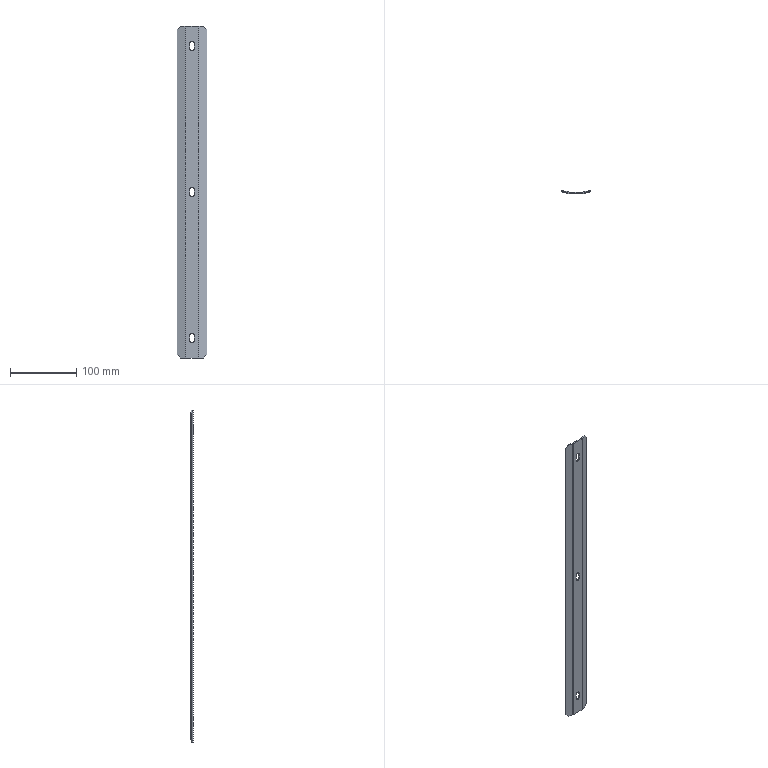Part | STEP file | SYL_0392D6J1SYL0380DJ1006_2_5-2 | 1 solid | 44 faces | box 44 x 4.447 x 500 mm | volume 32801 mm3 | plane 28 | cylinder 16 | commonest cylinder face diameters 7 x14 4 x2
STEP:
#1=CARTESIAN_POINT('',(-3.5,0.,-216.5));
#2=VERTEX_POINT('',#1);
#3=CARTESIAN_POINT('',(-3.5,1.5,-216.5));
#4=VERTEX_POINT('',#3);
#5=CARTESIAN_POINT('',(-3.5,1.5,-216.5));
#6=DIRECTION('',(0.,1.,0.));
#7=VECTOR('',#6,1000.);
#8=LINE('',#5,#7);
#9=EDGE_CURVE('',#2,#4,#8,.T.);
#10=ORIENTED_EDGE('',*,*,#9,.F.);
#11=CARTESIAN_POINT('',(-3.5,0.,-223.5));
#12=VERTEX_POINT('',#11);
#13=CARTESIAN_POINT('',(-3.5,0.,-250.));
#14=DIRECTION('',(0.,0.,-1.));
#15=VECTOR('',#14,1000.);
#16=LINE('',#13,#15);
#17=EDGE_CURVE('',#2,#12,#16,.T.);
#18=ORIENTED_EDGE('',*,*,#17,.T.);
#19=CARTESIAN_POINT('',(-3.5,1.5,-223.5));
#20=VERTEX_POINT('',#19);
#21=CARTESIAN_POINT('',(-3.5,1.5,-223.5));
#22=DIRECTION('',(0.,1.,0.));
#23=VECTOR('',#22,1000.);
#24=LINE('',#21,#23);
#25=EDGE_CURVE('',#12,#20,#24,.T.);
#26=ORIENTED_EDGE('',*,*,#25,.T.);
#27=CARTESIAN_POINT('',(-3.5,1.5,-216.5));
#28=DIRECTION('',(0.,0.,-1.));
#29=VECTOR('',#28,1000.);
#30=LINE('',#27,#29);
#31=EDGE_CURVE('',#4,#20,#30,.T.);
#32=ORIENTED_EDGE('',*,*,#31,.F.);
#33=EDGE_LOOP('',(#10,#18,#26,#32));
#34=FACE_OUTER_BOUND('',#33,.T.);
#35=CARTESIAN_POINT('',(-3.5,1.5,-216.5));
#36=DIRECTION('',(-1.,0.,0.));
#37=DIRECTION('',(0.,0.,-1.));
#38=AXIS2_PLACEMENT_3D('',#35,#36,#37);
#39=PLANE('',#38);
#40=ADVANCED_FACE('',(#34),#39,.F.);
#41=ORIENTED_EDGE('',*,*,#25,.F.);
#42=CARTESIAN_POINT('',(0.,0.,-227.));
#43=VERTEX_POINT('',#42);
#44=CARTESIAN_POINT('',(0.,0.,-223.5));
#45=DIRECTION('',(0.,-1.,0.));
#46=DIRECTION('',(0.,0.,-1.));
#47=AXIS2_PLACEMENT_3D('',#44,#45,#46);
#48=CIRCLE('',#47,3.5);
#49=EDGE_CURVE('',#12,#43,#48,.T.);
#50=ORIENTED_EDGE('',*,*,#49,.T.);
#51=CARTESIAN_POINT('',(0.,1.5,-227.));
#52=VERTEX_POINT('',#51);
#53=CARTESIAN_POINT('',(0.,1.5,-227.));
#54=DIRECTION('',(0.,1.,0.));
#55=VECTOR('',#54,1000.);
#56=LINE('',#53,#55);
#57=EDGE_CURVE('',#43,#52,#56,.T.);
#58=ORIENTED_EDGE('',*,*,#57,.T.);
#59=CARTESIAN_POINT('',(0.,1.5,-223.5));
#60=DIRECTION('',(0.,-1.,0.));
#61=DIRECTION('',(-1.,0.,0.));
#62=AXIS2_PLACEMENT_3D('',#59,#60,#61);
#63=CIRCLE('',#62,3.5);
#64=EDGE_CURVE('',#20,#52,#63,.T.);
#65=ORIENTED_EDGE('',*,*,#64,.F.);
#66=EDGE_LOOP('',(#41,#50,#58,#65));
#67=FACE_OUTER_BOUND('',#66,.T.);
#68=CARTESIAN_POINT('',(0.,1.5,-223.5));
#69=DIRECTION('',(0.,-1.,0.));
#70=DIRECTION('',(0.,0.,-1.));
#71=AXIS2_PLACEMENT_3D('',#68,#69,#70);
#72=CYLINDRICAL_SURFACE('',#71,3.5);
#73=ADVANCED_FACE('',(#67),#72,.F.);
#74=ORIENTED_EDGE('',*,*,#57,.F.);
#75=CARTESIAN_POINT('',(3.5,0.,-223.5));
#76=VERTEX_POINT('',#75);
#77=CARTESIAN_POINT('',(0.,0.,-223.5));
#78=DIRECTION('',(0.,-1.,0.));
#79=DIRECTION('',(0.,0.,-1.));
#80=AXIS2_PLACEMENT_3D('',#77,#78,#79);
#81=CIRCLE('',#80,3.5);
#82=EDGE_CURVE('',#43,#76,#81,.T.);
#83=ORIENTED_EDGE('',*,*,#82,.T.);
#84=CARTESIAN_POINT('',(3.5,1.5,-223.5));
#85=VERTEX_POINT('',#84);
#86=CARTESIAN_POINT('',(3.5,1.5,-223.5));
#87=DIRECTION('',(0.,1.,0.));
#88=VECTOR('',#87,1000.);
#89=LINE('',#86,#88);
#90=EDGE_CURVE('',#76,#85,#89,.T.);
#91=ORIENTED_EDGE('',*,*,#90,.T.);
#92=CARTESIAN_POINT('',(0.,1.5,-223.5));
#93=DIRECTION('',(0.,-1.,0.));
#94=DIRECTION('',(0.,0.,-1.));
#95=AXIS2_PLACEMENT_3D('',#92,#93,#94);
#96=CIRCLE('',#95,3.5);
#97=EDGE_CURVE('',#52,#85,#96,.T.);
#98=ORIENTED_EDGE('',*,*,#97,.F.);
#99=EDGE_LOOP('',(#74,#83,#91,#98));
#100=FACE_OUTER_BOUND('',#99,.T.);
#101=CARTESIAN_POINT('',(0.,1.5,-223.5));
#102=DIRECTION('',(0.,-1.,0.));
#103=DIRECTION('',(0.,0.,-1.));
#104=AXIS2_PLACEMENT_3D('',#101,#102,#103);
#105=CYLINDRICAL_SURFACE('',#104,3.5);
#106=ADVANCED_FACE('',(#100),#105,.F.);
#107=ORIENTED_EDGE('',*,*,#90,.F.);
#108=CARTESIAN_POINT('',(3.5,0.,-216.5));
#109=VERTEX_POINT('',#108);
#110=CARTESIAN_POINT('',(3.5,0.,-250.));
#111=DIRECTION('',(0.,0.,1.));
#112=VECTOR('',#111,1000.);
#113=LINE('',#110,#112);
#114=EDGE_CURVE('',#76,#109,#113,.T.);
#115=ORIENTED_EDGE('',*,*,#114,.T.);
#116=CARTESIAN_POINT('',(3.5,1.5,-216.5));
#117=VERTEX_POINT('',#116);
#118=CARTESIAN_POINT('',(3.5,1.5,-216.5));
#119=DIRECTION('',(0.,1.,0.));
#120=VECTOR('',#119,1000.);
#121=LINE('',#118,#120);
#122=EDGE_CURVE('',#109,#117,#121,.T.);
#123=ORIENTED_EDGE('',*,*,#122,.T.);
#124=CARTESIAN_POINT('',(3.5,1.5,-223.5));
#125=DIRECTION('',(0.,0.,1.));
#126=VECTOR('',#125,1000.);
#127=LINE('',#124,#126);
#128=EDGE_CURVE('',#85,#117,#127,.T.);
#129=ORIENTED_EDGE('',*,*,#128,.F.);
#130=EDGE_LOOP('',(#107,#115,#123,#129));
#131=FACE_OUTER_BOUND('',#130,.T.);
#132=CARTESIAN_POINT('',(3.5,1.5,-223.5));
#133=DIRECTION('',(1.,0.,0.));
#134=DIRECTION('',(0.,0.,1.));
#135=AXIS2_PLACEMENT_3D('',#132,#133,#134);
#136=PLANE('',#135);
#137=ADVANCED_FACE('',(#131),#136,.F.);
#138=ORIENTED_EDGE('',*,*,#122,.F.);
#139=CARTESIAN_POINT('',(0.,0.,-213.));
#140=VERTEX_POINT('',#139);
#141=CARTESIAN_POINT('',(0.,0.,-216.5));
#142=DIRECTION('',(0.,-1.,0.));
#143=DIRECTION('',(0.,0.,-1.));
#144=AXIS2_PLACEMENT_3D('',#141,#142,#143);
#145=CIRCLE('',#144,3.5);
#146=EDGE_CURVE('',#109,#140,#145,.T.);
#147=ORIENTED_EDGE('',*,*,#146,.T.);
#148=CARTESIAN_POINT('',(0.,1.5,-213.));
#149=VERTEX_POINT('',#148);
#150=CARTESIAN_POINT('',(0.,1.5,-213.));
#151=DIRECTION('',(0.,1.,0.));
#152=VECTOR('',#151,1000.);
#153=LINE('',#150,#152);
#154=EDGE_CURVE('',#140,#149,#153,.T.);
#155=ORIENTED_EDGE('',*,*,#154,.T.);
#156=CARTESIAN_POINT('',(0.,1.5,-216.5));
#157=DIRECTION('',(0.,-1.,0.));
#158=DIRECTION('',(1.,0.,0.));
#159=AXIS2_PLACEMENT_3D('',#156,#157,#158);
#160=CIRCLE('',#159,3.5);
#161=EDGE_CURVE('',#117,#149,#160,.T.);
#162=ORIENTED_EDGE('',*,*,#161,.F.);
#163=EDGE_LOOP('',(#138,#147,#155,#162));
#164=FACE_OUTER_BOUND('',#163,.T.);
#165=CARTESIAN_POINT('',(0.,1.5,-216.5));
#166=DIRECTION('',(0.,-1.,0.));
#167=DIRECTION('',(0.,0.,-1.));
#168=AXIS2_PLACEMENT_3D('',#165,#166,#167);
#169=CYLINDRICAL_SURFACE('',#168,3.5);
#170=ADVANCED_FACE('',(#164),#169,.F.);
#171=CARTESIAN_POINT('',(-3.5,0.,3.5));
#172=VERTEX_POINT('',#171);
#173=CARTESIAN_POINT('',(-3.5,1.5,3.5));
#174=VERTEX_POINT('',#173);
#175=CARTESIAN_POINT('',(-3.5,1.5,3.5));
#176=DIRECTION('',(0.,1.,0.));
#177=VECTOR('',#176,1000.);
#178=LINE('',#175,#177);
#179=EDGE_CURVE('',#172,#174,#178,.T.);
#180=ORIENTED_EDGE('',*,*,#179,.F.);
#181=CARTESIAN_POINT('',(-3.5,0.,-3.5));
#182=VERTEX_POINT('',#181);
#183=CARTESIAN_POINT('',(-3.5,0.,-250.));
#184=DIRECTION('',(0.,0.,-1.));
#185=VECTOR('',#184,1000.);
#186=LINE('',#183,#185);
#187=EDGE_CURVE('',#172,#182,#186,.T.);
#188=ORIENTED_EDGE('',*,*,#187,.T.);
#189=CARTESIAN_POINT('',(-3.5,1.5,-3.5));
#190=VERTEX_POINT('',#189);
#191=CARTESIAN_POINT('',(-3.5,1.5,-3.5));
#192=DIRECTION('',(0.,1.,0.));
#193=VECTOR('',#192,1000.);
#194=LINE('',#191,#193);
#195=EDGE_CURVE('',#182,#190,#194,.T.);
#196=ORIENTED_EDGE('',*,*,#195,.T.);
#197=CARTESIAN_POINT('',(-3.5,1.5,3.5));
#198=DIRECTION('',(0.,0.,-1.));
#199=VECTOR('',#198,1000.);
#200=LINE('',#197,#199);
#201=EDGE_CURVE('',#174,#190,#200,.T.);
#202=ORIENTED_EDGE('',*,*,#201,.F.);
#203=EDGE_LOOP('',(#180,#188,#196,#202));
#204=FACE_OUTER_BOUND('',#203,.T.);
#205=CARTESIAN_POINT('',(-3.5,1.5,3.5));
#206=DIRECTION('',(-1.,0.,0.));
#207=DIRECTION('',(0.,0.,-1.));
#208=AXIS2_PLACEMENT_3D('',#205,#206,#207);
#209=PLANE('',#208);
#210=ADVANCED_FACE('',(#204),#209,.F.);
#211=ORIENTED_EDGE('',*,*,#195,.F.);
#212=CARTESIAN_POINT('',(0.,0.,-7.));
#213=VERTEX_POINT('',#212);
#214=CARTESIAN_POINT('',(0.,0.,-3.5));
#215=DIRECTION('',(0.,-1.,0.));
#216=DIRECTION('',(0.,0.,-1.));
#217=AXIS2_PLACEMENT_3D('',#214,#215,#216);
#218=CIRCLE('',#217,3.5);
#219=EDGE_CURVE('',#182,#213,#218,.T.);
#220=ORIENTED_EDGE('',*,*,#219,.T.);
#221=CARTESIAN_POINT('',(0.,1.5,-7.));
#222=VERTEX_POINT('',#221);
#223=CARTESIAN_POINT('',(0.,1.5,-7.));
#224=DIRECTION('',(0.,1.,0.));
#225=VECTOR('',#224,1000.);
#226=LINE('',#223,#225);
#227=EDGE_CURVE('',#213,#222,#226,.T.);
#228=ORIENTED_EDGE('',*,*,#227,.T.);
#229=CARTESIAN_POINT('',(0.,1.5,-3.5));
#230=DIRECTION('',(0.,-1.,0.));
#231=DIRECTION('',(-1.,0.,0.));
#232=AXIS2_PLACEMENT_3D('',#229,#230,#231);
#233=CIRCLE('',#232,3.5);
#234=EDGE_CURVE('',#190,#222,#233,.T.);
#235=ORIENTED_EDGE('',*,*,#234,.F.);
#236=EDGE_LOOP('',(#211,#220,#228,#235));
#237=FACE_OUTER_BOUND('',#236,.T.);
#238=CARTESIAN_POINT('',(0.,1.5,-3.5));
#239=DIRECTION('',(0.,-1.,0.));
#240=DIRECTION('',(0.,0.,-1.));
#241=AXIS2_PLACEMENT_3D('',#238,#239,#240);
#242=CYLINDRICAL_SURFACE('',#241,3.5);
#243=ADVANCED_FACE('',(#237),#242,.F.);
#244=ORIENTED_EDGE('',*,*,#227,.F.);
#245=CARTESIAN_POINT('',(3.5,0.,-3.5));
#246=VERTEX_POINT('',#245);
#247=CARTESIAN_POINT('',(0.,0.,-3.5));
#248=DIRECTION('',(0.,-1.,0.));
#249=DIRECTION('',(0.,0.,-1.));
#250=AXIS2_PLACEMENT_3D('',#247,#248,#249);
#251=CIRCLE('',#250,3.5);
#252=EDGE_CURVE('',#213,#246,#251,.T.);
#253=ORIENTED_EDGE('',*,*,#252,.T.);
#254=CARTESIAN_POINT('',(3.5,1.5,-3.5));
#255=VERTEX_POINT('',#254);
#256=CARTESIAN_POINT('',(3.5,1.5,-3.5));
#257=DIRECTION('',(0.,1.,0.));
#258=VECTOR('',#257,1000.);
#259=LINE('',#256,#258);
#260=EDGE_CURVE('',#246,#255,#259,.T.);
#261=ORIENTED_EDGE('',*,*,#260,.T.);
#262=CARTESIAN_POINT('',(0.,1.5,-3.5));
#263=DIRECTION('',(0.,-1.,0.));
#264=DIRECTION('',(0.,0.,-1.));
#265=AXIS2_PLACEMENT_3D('',#262,#263,#264);
#266=CIRCLE('',#265,3.5);
#267=EDGE_CURVE('',#222,#255,#266,.T.);
#268=ORIENTED_EDGE('',*,*,#267,.F.);
#269=EDGE_LOOP('',(#244,#253,#261,#268));
#270=FACE_OUTER_BOUND('',#269,.T.);
#271=CARTESIAN_POINT('',(0.,1.5,-3.5));
#272=DIRECTION('',(0.,-1.,0.));
#273=DIRECTION('',(0.,0.,-1.));
#274=AXIS2_PLACEMENT_3D('',#271,#272,#273);
#275=CYLINDRICAL_SURFACE('',#274,3.5);
#276=ADVANCED_FACE('',(#270),#275,.F.);
#277=ORIENTED_EDGE('',*,*,#260,.F.);
#278=CARTESIAN_POINT('',(3.5,0.,3.5));
#279=VERTEX_POINT('',#278);
#280=CARTESIAN_POINT('',(3.5,0.,-250.));
#281=DIRECTION('',(0.,0.,1.));
#282=VECTOR('',#281,1000.);
#283=LINE('',#280,#282);
#284=EDGE_CURVE('',#246,#279,#283,.T.);
#285=ORIENTED_EDGE('',*,*,#284,.T.);
#286=CARTESIAN_POINT('',(3.5,1.5,3.5));
#287=VERTEX_POINT('',#286);
#288=CARTESIAN_POINT('',(3.5,1.5,3.5));
#289=DIRECTION('',(0.,1.,0.));
#290=VECTOR('',#289,1000.);
#291=LINE('',#288,#290);
#292=EDGE_CURVE('',#279,#287,#291,.T.);
#293=ORIENTED_EDGE('',*,*,#292,.T.);
#294=CARTESIAN_POINT('',(3.5,1.5,-3.5));
#295=DIRECTION('',(0.,0.,1.));
#296=VECTOR('',#295,1000.);
#297=LINE('',#294,#296);
#298=EDGE_CURVE('',#255,#287,#297,.T.);
#299=ORIENTED_EDGE('',*,*,#298,.F.);
#300=EDGE_LOOP('',(#277,#285,#293,#299));
#301=FACE_OUTER_BOUND('',#300,.T.);
#302=CARTESIAN_POINT('',(3.5,1.5,-3.5));
#303=DIRECTION('',(1.,0.,0.));
#304=DIRECTION('',(0.,0.,1.));
#305=AXIS2_PLACEMENT_3D('',#302,#303,#304);
#306=PLANE('',#305);
#307=ADVANCED_FACE('',(#301),#306,.F.);
#308=ORIENTED_EDGE('',*,*,#292,.F.);
#309=CARTESIAN_POINT('',(0.,0.,7.));
#310=VERTEX_POINT('',#309);
#311=CARTESIAN_POINT('',(0.,0.,3.5));
#312=DIRECTION('',(0.,-1.,0.));
#313=DIRECTION('',(0.,0.,-1.));
#314=AXIS2_PLACEMENT_3D('',#311,#312,#313);
#315=CIRCLE('',#314,3.5);
#316=EDGE_CURVE('',#279,#310,#315,.T.);
#317=ORIENTED_EDGE('',*,*,#316,.T.);
#318=CARTESIAN_POINT('',(0.,1.5,7.));
#319=VERTEX_POINT('',#318);
#320=CARTESIAN_POINT('',(0.,1.5,7.));
#321=DIRECTION('',(0.,1.,0.));
#322=VECTOR('',#321,1000.);
#323=LINE('',#320,#322);
#324=EDGE_CURVE('',#310,#319,#323,.T.);
#325=ORIENTED_EDGE('',*,*,#324,.T.);
#326=CARTESIAN_POINT('',(0.,1.5,3.5));
#327=DIRECTION('',(0.,-1.,0.));
#328=DIRECTION('',(1.,0.,0.));
#329=AXIS2_PLACEMENT_3D('',#326,#327,#328);
#330=CIRCLE('',#329,3.5);
#331=EDGE_CURVE('',#287,#319,#330,.T.);
#332=ORIENTED_EDGE('',*,*,#331,.F.);
#333=EDGE_LOOP('',(#308,#317,#325,#332));
#334=FACE_OUTER_BOUND('',#333,.T.);
#335=CARTESIAN_POINT('',(0.,1.5,3.5));
#336=DIRECTION('',(0.,-1.,0.));
#337=DIRECTION('',(0.,0.,-1.));
#338=AXIS2_PLACEMENT_3D('',#335,#336,#337);
#339=CYLINDRICAL_SURFACE('',#338,3.5);
#340=ADVANCED_FACE('',(#334),#339,.F.);
#341=CARTESIAN_POINT('',(-3.5,0.,223.5));
#342=VERTEX_POINT('',#341);
#343=CARTESIAN_POINT('',(-3.5,1.5,223.5));
#344=VERTEX_POINT('',#343);
#345=CARTESIAN_POINT('',(-3.5,1.5,223.5));
#346=DIRECTION('',(0.,1.,0.));
#347=VECTOR('',#346,1000.);
#348=LINE('',#345,#347);
#349=EDGE_CURVE('',#342,#344,#348,.T.);
#350=ORIENTED_EDGE('',*,*,#349,.F.);
#351=CARTESIAN_POINT('',(-3.5,0.,216.5));
#352=VERTEX_POINT('',#351);
#353=CARTESIAN_POINT('',(-3.5,0.,-250.));
#354=DIRECTION('',(0.,0.,-1.));
#355=VECTOR('',#354,1000.);
#356=LINE('',#353,#355);
#357=EDGE_CURVE('',#342,#352,#356,.T.);
#358=ORIENTED_EDGE('',*,*,#357,.T.);
#359=CARTESIAN_POINT('',(-3.5,1.5,216.5));
#360=VERTEX_POINT('',#359);
#361=CARTESIAN_POINT('',(-3.5,1.5,216.5));
#362=DIRECTION('',(0.,1.,0.));
#363=VECTOR('',#362,1000.);
#364=LINE('',#361,#363);
#365=EDGE_CURVE('',#352,#360,#364,.T.);
#366=ORIENTED_EDGE('',*,*,#365,.T.);
#367=CARTESIAN_POINT('',(-3.5,1.5,223.5));
#368=DIRECTION('',(0.,0.,-1.));
#369=VECTOR('',#368,1000.);
#370=LINE('',#367,#369);
#371=EDGE_CURVE('',#344,#360,#370,.T.);
#372=ORIENTED_EDGE('',*,*,#371,.F.);
#373=EDGE_LOOP('',(#350,#358,#366,#372));
#374=FACE_OUTER_BOUND('',#373,.T.);
#375=CARTESIAN_POINT('',(-3.5,1.5,223.5));
#376=DIRECTION('',(-1.,0.,0.));
#377=DIRECTION('',(0.,0.,-1.));
#378=AXIS2_PLACEMENT_3D('',#375,#376,#377);
#379=PLANE('',#378);
#380=ADVANCED_FACE('',(#374),#379,.F.);
#381=ORIENTED_EDGE('',*,*,#365,.F.);
#382=CARTESIAN_POINT('',(0.,0.,213.));
#383=VERTEX_POINT('',#382);
#384=CARTESIAN_POINT('',(0.,0.,216.5));
#385=DIRECTION('',(0.,-1.,0.));
#386=DIRECTION('',(0.,0.,-1.));
#387=AXIS2_PLACEMENT_3D('',#384,#385,#386);
#388=CIRCLE('',#387,3.5);
#389=EDGE_CURVE('',#352,#383,#388,.T.);
#390=ORIENTED_EDGE('',*,*,#389,.T.);
#391=CARTESIAN_POINT('',(0.,1.5,213.));
#392=VERTEX_POINT('',#391);
#393=CARTESIAN_POINT('',(0.,1.5,213.));
#394=DIRECTION('',(0.,1.,0.));
#395=VECTOR('',#394,1000.);
#396=LINE('',#393,#395);
#397=EDGE_CURVE('',#383,#392,#396,.T.);
#398=ORIENTED_EDGE('',*,*,#397,.T.);
#399=CARTESIAN_POINT('',(0.,1.5,216.5));
#400=DIRECTION('',(0.,-1.,0.));
#401=DIRECTION('',(-1.,0.,0.));
#402=AXIS2_PLACEMENT_3D('',#399,#400,#401);
#403=CIRCLE('',#402,3.5);
#404=EDGE_CURVE('',#360,#392,#403,.T.);
#405=ORIENTED_EDGE('',*,*,#404,.F.);
#406=EDGE_LOOP('',(#381,#390,#398,#405));
#407=FACE_OUTER_BOUND('',#406,.T.);
#408=CARTESIAN_POINT('',(0.,1.5,216.5));
#409=DIRECTION('',(0.,-1.,0.));
#410=DIRECTION('',(0.,0.,-1.));
#411=AXIS2_PLACEMENT_3D('',#408,#409,#410);
#412=CYLINDRICAL_SURFACE('',#411,3.5);
#413=ADVANCED_FACE('',(#407),#412,.F.);
#414=ORIENTED_EDGE('',*,*,#397,.F.);
#415=CARTESIAN_POINT('',(3.5,0.,216.5));
#416=VERTEX_POINT('',#415);
#417=CARTESIAN_POINT('',(0.,0.,216.5));
#418=DIRECTION('',(0.,-1.,0.));
#419=DIRECTION('',(0.,0.,-1.));
#420=AXIS2_PLACEMENT_3D('',#417,#418,#419);
#421=CIRCLE('',#420,3.5);
#422=EDGE_CURVE('',#383,#416,#421,.T.);
#423=ORIENTED_EDGE('',*,*,#422,.T.);
#424=CARTESIAN_POINT('',(3.5,1.5,216.5));
#425=VERTEX_POINT('',#424);
#426=CARTESIAN_POINT('',(3.5,1.5,216.5));
#427=DIRECTION('',(0.,1.,0.));
#428=VECTOR('',#427,1000.);
#429=LINE('',#426,#428);
#430=EDGE_CURVE('',#416,#425,#429,.T.);
#431=ORIENTED_EDGE('',*,*,#430,.T.);
#432=CARTESIAN_POINT('',(0.,1.5,216.5));
#433=DIRECTION('',(0.,-1.,0.));
#434=DIRECTION('',(0.,0.,-1.));
#435=AXIS2_PLACEMENT_3D('',#432,#433,#434);
#436=CIRCLE('',#435,3.5);
#437=EDGE_CURVE('',#392,#425,#436,.T.);
#438=ORIENTED_EDGE('',*,*,#437,.F.);
#439=EDGE_LOOP('',(#414,#423,#431,#438));
#440=FACE_OUTER_BOUND('',#439,.T.);
#441=CARTESIAN_POINT('',(0.,1.5,216.5));
#442=DIRECTION('',(0.,-1.,0.));
#443=DIRECTION('',(0.,0.,-1.));
#444=AXIS2_PLACEMENT_3D('',#441,#442,#443);
#445=CYLINDRICAL_SURFACE('',#444,3.5);
#446=ADVANCED_FACE('',(#440),#445,.F.);
#447=ORIENTED_EDGE('',*,*,#430,.F.);
#448=CARTESIAN_POINT('',(3.5,0.,223.5));
#449=VERTEX_POINT('',#448);
#450=CARTESIAN_POINT('',(3.5,0.,-250.));
#451=DIRECTION('',(0.,0.,1.));
#452=VECTOR('',#451,1000.);
#453=LINE('',#450,#452);
#454=EDGE_CURVE('',#416,#449,#453,.T.);
#455=ORIENTED_EDGE('',*,*,#454,.T.);
#456=CARTESIAN_POINT('',(3.5,1.5,223.5));
#457=VERTEX_POINT('',#456);
#458=CARTESIAN_POINT('',(3.5,1.5,223.5));
#459=DIRECTION('',(0.,1.,0.));
#460=VECTOR('',#459,1000.);
#461=LINE('',#458,#460);
#462=EDGE_CURVE('',#449,#457,#461,.T.);
#463=ORIENTED_EDGE('',*,*,#462,.T.);
#464=CARTESIAN_POINT('',(3.5,1.5,216.5));
#465=DIRECTION('',(0.,0.,1.));
#466=VECTOR('',#465,1000.);
#467=LINE('',#464,#466);
#468=EDGE_CURVE('',#425,#457,#467,.T.);
#469=ORIENTED_EDGE('',*,*,#468,.F.);
#470=EDGE_LOOP('',(#447,#455,#463,#469));
#471=FACE_OUTER_BOUND('',#470,.T.);
#472=CARTESIAN_POINT('',(3.5,1.5,216.5));
#473=DIRECTION('',(1.,0.,0.));
#474=DIRECTION('',(0.,0.,1.));
#475=AXIS2_PLACEMENT_3D('',#472,#473,#474);
#476=PLANE('',#475);
#477=ADVANCED_FACE('',(#471),#476,.F.);
#478=ORIENTED_EDGE('',*,*,#462,.F.);
#479=CARTESIAN_POINT('',(0.,0.,227.));
#480=VERTEX_POINT('',#479);
#481=CARTESIAN_POINT('',(0.,0.,223.5));
#482=DIRECTION('',(0.,-1.,0.));
#483=DIRECTION('',(0.,0.,-1.));
#484=AXIS2_PLACEMENT_3D('',#481,#482,#483);
#485=CIRCLE('',#484,3.5);
#486=EDGE_CURVE('',#449,#480,#485,.T.);
#487=ORIENTED_EDGE('',*,*,#486,.T.);
#488=CARTESIAN_POINT('',(0.,1.5,227.));
#489=VERTEX_POINT('',#488);
#490=CARTESIAN_POINT('',(0.,1.5,227.));
#491=DIRECTION('',(0.,1.,0.));
#492=VECTOR('',#491,1000.);
#493=LINE('',#490,#492);
#494=EDGE_CURVE('',#480,#489,#493,.T.);
#495=ORIENTED_EDGE('',*,*,#494,.T.);
#496=CARTESIAN_POINT('',(0.,1.5,223.5));
#497=DIRECTION('',(0.,-1.,0.));
#498=DIRECTION('',(1.,0.,0.));
#499=AXIS2_PLACEMENT_3D('',#496,#497,#498);
#500=CIRCLE('',#499,3.5);
#501=EDGE_CURVE('',#457,#489,#500,.T.);
#502=ORIENTED_EDGE('',*,*,#501,.F.);
#503=EDGE_LOOP('',(#478,#487,#495,#502));
#504=FACE_OUTER_BOUND('',#503,.T.);
#505=CARTESIAN_POINT('',(0.,1.5,223.5));
#506=DIRECTION('',(0.,-1.,0.));
#507=DIRECTION('',(0.,0.,-1.));
#508=AXIS2_PLACEMENT_3D('',#505,#506,#507);
#509=CYLINDRICAL_SURFACE('',#508,3.5);
#510=ADVANCED_FACE('',(#504),#509,.F.);
#511=CARTESIAN_POINT('',(-17.149,1.782,-250.));
#512=VERTEX_POINT('',#511);
#513=CARTESIAN_POINT('',(-16.786,3.238,-250.));
#514=VERTEX_POINT('',#513);
#515=CARTESIAN_POINT('',(-16.786,3.238,-250.));
#516=DIRECTION('',(0.2419,0.9703,0.));
#517=VECTOR('',#516,1000.);
#518=LINE('',#515,#517);
#519=EDGE_CURVE('',#512,#514,#518,.T.);
#520=ORIENTED_EDGE('',*,*,#519,.F.);
#521=CARTESIAN_POINT('',(-22.,2.992,-245.));
#522=VERTEX_POINT('',#521);
#523=CARTESIAN_POINT('',(-17.149,1.782,-250.));
#524=DIRECTION('',(-0.6861,0.1711,0.7071));
#525=VECTOR('',#524,1000.);
#526=LINE('',#523,#525);
#527=EDGE_CURVE('',#512,#522,#526,.T.);
#528=ORIENTED_EDGE('',*,*,#527,.T.);
#529=CARTESIAN_POINT('',(-21.637,4.447,-245.));
#530=VERTEX_POINT('',#529);
#531=CARTESIAN_POINT('',(-21.637,4.447,-245.));
#532=DIRECTION('',(0.2419,0.9703,0.));
#533=VECTOR('',#532,1000.);
#534=LINE('',#531,#533);
#535=EDGE_CURVE('',#522,#530,#534,.T.);
#536=ORIENTED_EDGE('',*,*,#535,.T.);
#537=CARTESIAN_POINT('',(-16.786,3.238,-250.));
#538=DIRECTION('',(-0.6861,0.1711,0.7071));
#539=VECTOR('',#538,1000.);
#540=LINE('',#537,#539);
#541=EDGE_CURVE('',#514,#530,#540,.T.);
#542=ORIENTED_EDGE('',*,*,#541,.F.);
#543=EDGE_LOOP('',(#520,#528,#536,#542));
#544=FACE_OUTER_BOUND('',#543,.T.);
#545=CARTESIAN_POINT('',(-16.786,3.238,-250.));
#546=DIRECTION('',(0.6861,-0.1711,0.7071));
#547=DIRECTION('',(-0.6861,0.1711,0.7071));
#548=AXIS2_PLACEMENT_3D('',#545,#546,#547);
#549=PLANE('',#548);
#550=ADVANCED_FACE('',(#544),#549,.F.);
#551=ORIENTED_EDGE('',*,*,#535,.F.);
#552=CARTESIAN_POINT('',(-22.,2.992,245.));
#553=VERTEX_POINT('',#552);
#554=CARTESIAN_POINT('',(-22.,2.992,-250.));
#555=DIRECTION('',(0.,0.,1.));
#556=VECTOR('',#555,1000.);
#557=LINE('',#554,#556);
#558=EDGE_CURVE('',#522,#553,#557,.T.);
#559=ORIENTED_EDGE('',*,*,#558,.T.);
#560=CARTESIAN_POINT('',(-21.637,4.447,245.));
#561=VERTEX_POINT('',#560);
#562=CARTESIAN_POINT('',(-21.637,4.447,245.));
#563=DIRECTION('',(0.2419,0.9703,0.));
#564=VECTOR('',#563,1000.);
#565=LINE('',#562,#564);
#566=EDGE_CURVE('',#553,#561,#565,.T.);
#567=ORIENTED_EDGE('',*,*,#566,.T.);
#568=CARTESIAN_POINT('',(-21.637,4.447,-245.));
#569=DIRECTION('',(0.,0.,1.));
#570=VECTOR('',#569,1000.);
#571=LINE('',#568,#570);
#572=EDGE_CURVE('',#530,#561,#571,.T.);
#573=ORIENTED_EDGE('',*,*,#572,.F.);
#574=EDGE_LOOP('',(#551,#559,#567,#573));
#575=FACE_OUTER_BOUND('',#574,.T.);
#576=CARTESIAN_POINT('',(-21.637,4.447,-245.));
#577=DIRECTION('',(0.9703,-0.2419,0.));
#578=DIRECTION('',(0.,0.,1.));
#579=AXIS2_PLACEMENT_3D('',#576,#577,#578);
#580=PLANE('',#579);
#581=ADVANCED_FACE('',(#575),#580,.F.);
#582=ORIENTED_EDGE('',*,*,#566,.F.);
#583=CARTESIAN_POINT('',(-17.149,1.782,250.));
#584=VERTEX_POINT('',#583);
#585=CARTESIAN_POINT('',(-22.,2.992,245.));
#586=DIRECTION('',(0.6861,-0.1711,0.7071));
#587=VECTOR('',#586,1000.);
#588=LINE('',#585,#587);
#589=EDGE_CURVE('',#553,#584,#588,.T.);
#590=ORIENTED_EDGE('',*,*,#589,.T.);
#591=CARTESIAN_POINT('',(-16.786,3.238,250.));
#592=VERTEX_POINT('',#591);
#593=CARTESIAN_POINT('',(-16.786,3.238,250.));
#594=DIRECTION('',(0.2419,0.9703,0.));
#595=VECTOR('',#594,1000.);
#596=LINE('',#593,#595);
#597=EDGE_CURVE('',#584,#592,#596,.T.);
#598=ORIENTED_EDGE('',*,*,#597,.T.);
#599=CARTESIAN_POINT('',(-21.637,4.447,245.));
#600=DIRECTION('',(0.6861,-0.1711,0.7071));
#601=VECTOR('',#600,1000.);
#602=LINE('',#599,#601);
#603=EDGE_CURVE('',#561,#592,#602,.T.);
#604=ORIENTED_EDGE('',*,*,#603,.F.);
#605=EDGE_LOOP('',(#582,#590,#598,#604));
#606=FACE_OUTER_BOUND('',#605,.T.);
#607=CARTESIAN_POINT('',(-21.637,4.447,245.));
#608=DIRECTION('',(0.6861,-0.1711,-0.7071));
#609=DIRECTION('',(0.6861,-0.1711,0.7071));
#610=AXIS2_PLACEMENT_3D('',#607,#608,#609);
#611=PLANE('',#610);
#612=ADVANCED_FACE('',(#606),#611,.F.);
#613=ORIENTED_EDGE('',*,*,#597,.F.);
#614=CARTESIAN_POINT('',(-10.417,0.104,250.));
#615=VERTEX_POINT('',#614);
#616=CARTESIAN_POINT('',(-22.,2.992,250.));
#617=DIRECTION('',(-0.9703,0.2419,0.));
#618=VECTOR('',#617,1000.);
#619=LINE('',#616,#618);
#620=EDGE_CURVE('',#615,#584,#619,.T.);
#621=ORIENTED_EDGE('',*,*,#620,.F.);
#622=CARTESIAN_POINT('',(-10.054,1.559,250.));
#623=VERTEX_POINT('',#622);
#624=CARTESIAN_POINT('',(-10.054,1.559,250.));
#625=DIRECTION('',(0.2419,0.9703,0.));
#626=VECTOR('',#625,1000.);
#627=LINE('',#624,#626);
#628=EDGE_CURVE('',#615,#623,#627,.T.);
#629=ORIENTED_EDGE('',*,*,#628,.T.);
#630=CARTESIAN_POINT('',(-10.054,1.559,250.));
#631=DIRECTION('',(-0.9703,0.2419,0.));
#632=VECTOR('',#631,1000.);
#633=LINE('',#630,#632);
#634=EDGE_CURVE('',#623,#592,#633,.T.);
#635=ORIENTED_EDGE('',*,*,#634,.T.);
#636=EDGE_LOOP('',(#613,#621,#629,#635));
#637=FACE_OUTER_BOUND('',#636,.T.);
#638=CARTESIAN_POINT('',(-10.054,1.559,250.));
#639=DIRECTION('',(0.,0.,1.));
#640=DIRECTION('',(-0.9703,0.2419,0.));
#641=AXIS2_PLACEMENT_3D('',#638,#639,#640);
#642=PLANE('',#641);
#643=ADVANCED_FACE('',(#637),#642,.T.);
#644=ORIENTED_EDGE('',*,*,#628,.F.);
#645=CARTESIAN_POINT('',(-9.57,0.,250.));
#646=VERTEX_POINT('',#645);
#647=CARTESIAN_POINT('',(-9.57,3.5,250.));
#648=DIRECTION('',(0.,0.,-1.));
#649=DIRECTION('',(1.,0.,0.));
#650=AXIS2_PLACEMENT_3D('',#647,#648,#649);
#651=CIRCLE('',#650,3.5);
#652=EDGE_CURVE('',#646,#615,#651,.T.);
#653=ORIENTED_EDGE('',*,*,#652,.F.);
#654=CARTESIAN_POINT('',(-9.57,1.5,250.));
#655=VERTEX_POINT('',#654);
#656=CARTESIAN_POINT('',(-9.57,1.5,250.));
#657=DIRECTION('',(0.,1.,0.));
#658=VECTOR('',#657,1000.);
#659=LINE('',#656,#658);
#660=EDGE_CURVE('',#646,#655,#659,.T.);
#661=ORIENTED_EDGE('',*,*,#660,.T.);
#662=CARTESIAN_POINT('',(-9.57,3.5,250.));
#663=DIRECTION('',(0.,0.,-1.));
#664=DIRECTION('',(0.,-1.,0.));
#665=AXIS2_PLACEMENT_3D('',#662,#663,#664);
#666=CIRCLE('',#665,2.);
#667=EDGE_CURVE('',#655,#623,#666,.T.);
#668=ORIENTED_EDGE('',*,*,#667,.T.);
#669=EDGE_LOOP('',(#644,#653,#661,#668));
#670=FACE_OUTER_BOUND('',#669,.T.);
#671=CARTESIAN_POINT('',(-9.57,3.5,250.));
#672=DIRECTION('',(0.,0.,1.));
#673=DIRECTION('',(1.,0.,0.));
#674=AXIS2_PLACEMENT_3D('',#671,#672,#673);
#675=PLANE('',#674);
#676=ADVANCED_FACE('',(#670),#675,.T.);
#677=ORIENTED_EDGE('',*,*,#660,.F.);
#678=CARTESIAN_POINT('',(9.57,0.,250.));
#679=VERTEX_POINT('',#678);
#680=CARTESIAN_POINT('',(-9.57,0.,250.));
#681=DIRECTION('',(1.,0.,0.));
#682=VECTOR('',#681,1000.);
#683=LINE('',#680,#682);
#684=EDGE_CURVE('',#646,#679,#683,.T.);
#685=ORIENTED_EDGE('',*,*,#684,.T.);
#686=CARTESIAN_POINT('',(9.57,1.5,250.));
#687=VERTEX_POINT('',#686);
#688=CARTESIAN_POINT('',(9.57,1.5,250.));
#689=DIRECTION('',(0.,1.,0.));
#690=VECTOR('',#689,1000.);
#691=LINE('',#688,#690);
#692=EDGE_CURVE('',#679,#687,#691,.T.);
#693=ORIENTED_EDGE('',*,*,#692,.T.);
#694=CARTESIAN_POINT('',(-9.57,1.5,250.));
#695=DIRECTION('',(1.,0.,0.));
#696=VECTOR('',#695,1000.);
#697=LINE('',#694,#696);
#698=EDGE_CURVE('',#655,#687,#697,.T.);
#699=ORIENTED_EDGE('',*,*,#698,.F.);
#700=EDGE_LOOP('',(#677,#685,#693,#699));
#701=FACE_OUTER_BOUND('',#700,.T.);
#702=CARTESIAN_POINT('',(-9.57,1.5,250.));
#703=DIRECTION('',(0.,0.,-1.));
#704=DIRECTION('',(1.,0.,0.));
#705=AXIS2_PLACEMENT_3D('',#702,#703,#704);
#706=PLANE('',#705);
#707=ADVANCED_FACE('',(#701),#706,.F.);
#708=ORIENTED_EDGE('',*,*,#692,.F.);
#709=CARTESIAN_POINT('',(10.417,0.104,250.));
#710=VERTEX_POINT('',#709);
#711=CARTESIAN_POINT('',(9.57,3.5,250.));
#712=DIRECTION('',(0.,0.,-1.));
#713=DIRECTION('',(1.,0.,0.));
#714=AXIS2_PLACEMENT_3D('',#711,#712,#713);
#715=CIRCLE('',#714,3.5);
#716=EDGE_CURVE('',#710,#679,#715,.T.);
#717=ORIENTED_EDGE('',*,*,#716,.F.);
#718=CARTESIAN_POINT('',(10.054,1.559,250.));
#719=VERTEX_POINT('',#718);
#720=CARTESIAN_POINT('',(10.054,1.559,250.));
#721=DIRECTION('',(-0.2419,0.9703,0.));
#722=VECTOR('',#721,1000.);
#723=LINE('',#720,#722);
#724=EDGE_CURVE('',#710,#719,#723,.T.);
#725=ORIENTED_EDGE('',*,*,#724,.T.);
#726=CARTESIAN_POINT('',(9.57,3.5,250.));
#727=DIRECTION('',(0.,0.,-1.));
#728=DIRECTION('',(0.2419,-0.9703,0.));
#729=AXIS2_PLACEMENT_3D('',#726,#727,#728);
#730=CIRCLE('',#729,2.);
#731=EDGE_CURVE('',#719,#687,#730,.T.);
#732=ORIENTED_EDGE('',*,*,#731,.T.);
#733=EDGE_LOOP('',(#708,#717,#725,#732));
#734=FACE_OUTER_BOUND('',#733,.T.);
#735=CARTESIAN_POINT('',(9.57,3.5,250.));
#736=DIRECTION('',(0.,0.,1.));
#737=DIRECTION('',(1.,0.,0.));
#738=AXIS2_PLACEMENT_3D('',#735,#736,#737);
#739=PLANE('',#738);
#740=ADVANCED_FACE('',(#734),#739,.T.);
#741=ORIENTED_EDGE('',*,*,#724,.F.);
#742=CARTESIAN_POINT('',(17.149,1.782,250.));
#743=VERTEX_POINT('',#742);
#744=CARTESIAN_POINT('',(10.417,0.104,250.));
#745=DIRECTION('',(-0.9703,-0.2419,0.));
#746=VECTOR('',#745,1000.);
#747=LINE('',#744,#746);
#748=EDGE_CURVE('',#743,#710,#747,.T.);
#749=ORIENTED_EDGE('',*,*,#748,.F.);
#750=CARTESIAN_POINT('',(16.786,3.238,250.));
#751=VERTEX_POINT('',#750);
#752=CARTESIAN_POINT('',(16.786,3.238,250.));
#753=DIRECTION('',(-0.2419,0.9703,0.));
#754=VECTOR('',#753,1000.);
#755=LINE('',#752,#754);
#756=EDGE_CURVE('',#743,#751,#755,.T.);
#757=ORIENTED_EDGE('',*,*,#756,.T.);
#758=CARTESIAN_POINT('',(16.786,3.238,250.));
#759=DIRECTION('',(-0.9703,-0.2419,0.));
#760=VECTOR('',#759,1000.);
#761=LINE('',#758,#760);
#762=EDGE_CURVE('',#751,#719,#761,.T.);
#763=ORIENTED_EDGE('',*,*,#762,.T.);
#764=EDGE_LOOP('',(#741,#749,#757,#763));
#765=FACE_OUTER_BOUND('',#764,.T.);
#766=CARTESIAN_POINT('',(16.786,3.238,250.));
#767=DIRECTION('',(0.,0.,1.));
#768=DIRECTION('',(-0.9703,-0.2419,0.));
#769=AXIS2_PLACEMENT_3D('',#766,#767,#768);
#770=PLANE('',#769);
#771=ADVANCED_FACE('',(#765),#770,.T.);
#772=ORIENTED_EDGE('',*,*,#756,.F.);
#773=CARTESIAN_POINT('',(22.,2.992,245.));
#774=VERTEX_POINT('',#773);
#775=CARTESIAN_POINT('',(17.149,1.782,250.));
#776=DIRECTION('',(0.6861,0.1711,-0.7071));
#777=VECTOR('',#776,1000.);
#778=LINE('',#775,#777);
#779=EDGE_CURVE('',#743,#774,#778,.T.);
#780=ORIENTED_EDGE('',*,*,#779,.T.);
#781=CARTESIAN_POINT('',(21.637,4.447,245.));
#782=VERTEX_POINT('',#781);
#783=CARTESIAN_POINT('',(21.637,4.447,245.));
#784=DIRECTION('',(-0.2419,0.9703,0.));
#785=VECTOR('',#784,1000.);
#786=LINE('',#783,#785);
#787=EDGE_CURVE('',#774,#782,#786,.T.);
#788=ORIENTED_EDGE('',*,*,#787,.T.);
#789=CARTESIAN_POINT('',(16.786,3.238,250.));
#790=DIRECTION('',(0.6861,0.1711,-0.7071));
#791=VECTOR('',#790,1000.);
#792=LINE('',#789,#791);
#793=EDGE_CURVE('',#751,#782,#792,.T.);
#794=ORIENTED_EDGE('',*,*,#793,.F.);
#795=EDGE_LOOP('',(#772,#780,#788,#794));
#796=FACE_OUTER_BOUND('',#795,.T.);
#797=CARTESIAN_POINT('',(16.786,3.238,250.));
#798=DIRECTION('',(-0.6861,-0.1711,-0.7071));
#799=DIRECTION('',(0.6861,0.1711,-0.7071));
#800=AXIS2_PLACEMENT_3D('',#797,#798,#799);
#801=PLANE('',#800);
#802=ADVANCED_FACE('',(#796),#801,.F.);
#803=ORIENTED_EDGE('',*,*,#787,.F.);
#804=CARTESIAN_POINT('',(22.,2.992,-245.));
#805=VERTEX_POINT('',#804);
#806=CARTESIAN_POINT('',(22.,2.992,-250.));
#807=DIRECTION('',(0.,0.,-1.));
#808=VECTOR('',#807,1000.);
#809=LINE('',#806,#808);
#810=EDGE_CURVE('',#774,#805,#809,.T.);
#811=ORIENTED_EDGE('',*,*,#810,.T.);
#812=CARTESIAN_POINT('',(21.637,4.447,-245.));
#813=VERTEX_POINT('',#812);
#814=CARTESIAN_POINT('',(21.637,4.447,-245.));
#815=DIRECTION('',(-0.2419,0.9703,0.));
#816=VECTOR('',#815,1000.);
#817=LINE('',#814,#816);
#818=EDGE_CURVE('',#805,#813,#817,.T.);
#819=ORIENTED_EDGE('',*,*,#818,.T.);
#820=CARTESIAN_POINT('',(21.637,4.447,245.));
#821=DIRECTION('',(0.,0.,-1.));
#822=VECTOR('',#821,1000.);
#823=LINE('',#820,#822);
#824=EDGE_CURVE('',#782,#813,#823,.T.);
#825=ORIENTED_EDGE('',*,*,#824,.F.);
#826=EDGE_LOOP('',(#803,#811,#819,#825));
#827=FACE_OUTER_BOUND('',#826,.T.);
#828=CARTESIAN_POINT('',(21.637,4.447,245.));
#829=DIRECTION('',(-0.9703,-0.2419,0.));
#830=DIRECTION('',(0.,0.,-1.));
#831=AXIS2_PLACEMENT_3D('',#828,#829,#830);
#832=PLANE('',#831);
#833=ADVANCED_FACE('',(#827),#832,.F.);
#834=ORIENTED_EDGE('',*,*,#818,.F.);
#835=CARTESIAN_POINT('',(17.149,1.782,-250.));
#836=VERTEX_POINT('',#835);
#837=CARTESIAN_POINT('',(22.,2.992,-245.));
#838=DIRECTION('',(-0.6861,-0.1711,-0.7071));
#839=VECTOR('',#838,1000.);
#840=LINE('',#837,#839);
#841=EDGE_CURVE('',#805,#836,#840,.T.);
#842=ORIENTED_EDGE('',*,*,#841,.T.);
#843=CARTESIAN_POINT('',(16.786,3.238,-250.));
#844=VERTEX_POINT('',#843);
#845=CARTESIAN_POINT('',(16.786,3.238,-250.));
#846=DIRECTION('',(-0.2419,0.9703,0.));
#847=VECTOR('',#846,1000.);
#848=LINE('',#845,#847);
#849=EDGE_CURVE('',#836,#844,#848,.T.);
#850=ORIENTED_EDGE('',*,*,#849,.T.);
#851=CARTESIAN_POINT('',(21.637,4.447,-245.));
#852=DIRECTION('',(-0.6861,-0.1711,-0.7071));
#853=VECTOR('',#852,1000.);
#854=LINE('',#851,#853);
#855=EDGE_CURVE('',#813,#844,#854,.T.);
#856=ORIENTED_EDGE('',*,*,#855,.F.);
#857=EDGE_LOOP('',(#834,#842,#850,#856));
#858=FACE_OUTER_BOUND('',#857,.T.);
#859=CARTESIAN_POINT('',(21.637,4.447,-245.));
#860=DIRECTION('',(-0.6861,-0.1711,0.7071));
#861=DIRECTION('',(-0.6861,-0.1711,-0.7071));
#862=AXIS2_PLACEMENT_3D('',#859,#860,#861);
#863=PLANE('',#862);
#864=ADVANCED_FACE('',(#858),#863,.F.);
#865=ORIENTED_EDGE('',*,*,#849,.F.);
#866=CARTESIAN_POINT('',(10.417,0.104,-250.));
#867=VERTEX_POINT('',#866);
#868=CARTESIAN_POINT('',(10.417,0.104,-250.));
#869=DIRECTION('',(0.9703,0.2419,0.));
#870=VECTOR('',#869,1000.);
#871=LINE('',#868,#870);
#872=EDGE_CURVE('',#867,#836,#871,.T.);
#873=ORIENTED_EDGE('',*,*,#872,.F.);
#874=CARTESIAN_POINT('',(10.054,1.559,-250.));
#875=VERTEX_POINT('',#874);
#876=CARTESIAN_POINT('',(10.054,1.559,-250.));
#877=DIRECTION('',(-0.2419,0.9703,0.));
#878=VECTOR('',#877,1000.);
#879=LINE('',#876,#878);
#880=EDGE_CURVE('',#867,#875,#879,.T.);
#881=ORIENTED_EDGE('',*,*,#880,.T.);
#882=CARTESIAN_POINT('',(10.054,1.559,-250.));
#883=DIRECTION('',(0.9703,0.2419,0.));
#884=VECTOR('',#883,1000.);
#885=LINE('',#882,#884);
#886=EDGE_CURVE('',#875,#844,#885,.T.);
#887=ORIENTED_EDGE('',*,*,#886,.T.);
#888=EDGE_LOOP('',(#865,#873,#881,#887));
#889=FACE_OUTER_BOUND('',#888,.T.);
#890=CARTESIAN_POINT('',(10.054,1.559,-250.));
#891=DIRECTION('',(0.,0.,-1.));
#892=DIRECTION('',(0.9703,0.2419,0.));
#893=AXIS2_PLACEMENT_3D('',#890,#891,#892);
#894=PLANE('',#893);
#895=ADVANCED_FACE('',(#889),#894,.T.);
#896=ORIENTED_EDGE('',*,*,#880,.F.);
#897=CARTESIAN_POINT('',(9.57,0.,-250.));
#898=VERTEX_POINT('',#897);
#899=CARTESIAN_POINT('',(9.57,3.5,-250.));
#900=DIRECTION('',(0.,0.,1.));
#901=DIRECTION('',(1.,0.,0.));
#902=AXIS2_PLACEMENT_3D('',#899,#900,#901);
#903=CIRCLE('',#902,3.5);
#904=EDGE_CURVE('',#898,#867,#903,.T.);
#905=ORIENTED_EDGE('',*,*,#904,.F.);
#906=CARTESIAN_POINT('',(9.57,1.5,-250.));
#907=VERTEX_POINT('',#906);
#908=CARTESIAN_POINT('',(9.57,1.5,-250.));
#909=DIRECTION('',(0.,1.,0.));
#910=VECTOR('',#909,1000.);
#911=LINE('',#908,#910);
#912=EDGE_CURVE('',#898,#907,#911,.T.);
#913=ORIENTED_EDGE('',*,*,#912,.T.);
#914=CARTESIAN_POINT('',(9.57,3.5,-250.));
#915=DIRECTION('',(0.,0.,1.));
#916=DIRECTION('',(0.,-1.,0.));
#917=AXIS2_PLACEMENT_3D('',#914,#915,#916);
#918=CIRCLE('',#917,2.);
#919=EDGE_CURVE('',#907,#875,#918,.T.);
#920=ORIENTED_EDGE('',*,*,#919,.T.);
#921=EDGE_LOOP('',(#896,#905,#913,#920));
#922=FACE_OUTER_BOUND('',#921,.T.);
#923=CARTESIAN_POINT('',(9.57,3.5,-250.));
#924=DIRECTION('',(0.,0.,-1.));
#925=DIRECTION('',(-1.,0.,0.));
#926=AXIS2_PLACEMENT_3D('',#923,#924,#925);
#927=PLANE('',#926);
#928=ADVANCED_FACE('',(#922),#927,.T.);
#929=ORIENTED_EDGE('',*,*,#912,.F.);
#930=CARTESIAN_POINT('',(-9.57,0.,-250.));
#931=VERTEX_POINT('',#930);
#932=CARTESIAN_POINT('',(-9.57,0.,-250.));
#933=DIRECTION('',(-1.,0.,0.));
#934=VECTOR('',#933,1000.);
#935=LINE('',#932,#934);
#936=EDGE_CURVE('',#898,#931,#935,.T.);
#937=ORIENTED_EDGE('',*,*,#936,.T.);
#938=CARTESIAN_POINT('',(-9.57,1.5,-250.));
#939=VERTEX_POINT('',#938);
#940=CARTESIAN_POINT('',(-9.57,1.5,-250.));
#941=DIRECTION('',(0.,1.,0.));
#942=VECTOR('',#941,1000.);
#943=LINE('',#940,#942);
#944=EDGE_CURVE('',#931,#939,#943,.T.);
#945=ORIENTED_EDGE('',*,*,#944,.T.);
#946=CARTESIAN_POINT('',(9.57,1.5,-250.));
#947=DIRECTION('',(-1.,0.,0.));
#948=VECTOR('',#947,1000.);
#949=LINE('',#946,#948);
#950=EDGE_CURVE('',#907,#939,#949,.T.);
#951=ORIENTED_EDGE('',*,*,#950,.F.);
#952=EDGE_LOOP('',(#929,#937,#945,#951));
#953=FACE_OUTER_BOUND('',#952,.T.);
#954=CARTESIAN_POINT('',(9.57,1.5,-250.));
#955=DIRECTION('',(0.,0.,1.));
#956=DIRECTION('',(-1.,0.,0.));
#957=AXIS2_PLACEMENT_3D('',#954,#955,#956);
#958=PLANE('',#957);
#959=ADVANCED_FACE('',(#953),#958,.F.);
#960=ORIENTED_EDGE('',*,*,#944,.F.);
#961=CARTESIAN_POINT('',(-10.417,0.104,-250.));
#962=VERTEX_POINT('',#961);
#963=CARTESIAN_POINT('',(-9.57,3.5,-250.));
#964=DIRECTION('',(0.,0.,1.));
#965=DIRECTION('',(1.,0.,0.));
#966=AXIS2_PLACEMENT_3D('',#963,#964,#965);
#967=CIRCLE('',#966,3.5);
#968=EDGE_CURVE('',#962,#931,#967,.T.);
#969=ORIENTED_EDGE('',*,*,#968,.F.);
#970=CARTESIAN_POINT('',(-10.054,1.559,-250.));
#971=VERTEX_POINT('',#970);
#972=CARTESIAN_POINT('',(-10.054,1.559,-250.));
#973=DIRECTION('',(0.2419,0.9703,0.));
#974=VECTOR('',#973,1000.);
#975=LINE('',#972,#974);
#976=EDGE_CURVE('',#962,#971,#975,.T.);
#977=ORIENTED_EDGE('',*,*,#976,.T.);
#978=CARTESIAN_POINT('',(-9.57,3.5,-250.));
#979=DIRECTION('',(0.,0.,1.));
#980=DIRECTION('',(-0.2419,-0.9703,0.));
#981=AXIS2_PLACEMENT_3D('',#978,#979,#980);
#982=CIRCLE('',#981,2.);
#983=EDGE_CURVE('',#971,#939,#982,.T.);
#984=ORIENTED_EDGE('',*,*,#983,.T.);
#985=EDGE_LOOP('',(#960,#969,#977,#984));
#986=FACE_OUTER_BOUND('',#985,.T.);
#987=CARTESIAN_POINT('',(-9.57,3.5,-250.));
#988=DIRECTION('',(0.,0.,-1.));
#989=DIRECTION('',(-1.,0.,0.));
#990=AXIS2_PLACEMENT_3D('',#987,#988,#989);
#991=PLANE('',#990);
#992=ADVANCED_FACE('',(#986),#991,.T.);
#993=CARTESIAN_POINT('',(0.,0.,223.5));
#994=DIRECTION('',(0.,-1.,0.));
#995=DIRECTION('',(0.,0.,-1.));
#996=AXIS2_PLACEMENT_3D('',#993,#994,#995);
#997=CIRCLE('',#996,3.5);
#998=EDGE_CURVE('',#480,#342,#997,.T.);
#999=ORIENTED_EDGE('',*,*,#998,.T.);
#1000=ORIENTED_EDGE('',*,*,#349,.T.);
#1001=CARTESIAN_POINT('',(0.,1.5,223.5));
#1002=DIRECTION('',(0.,-1.,0.));
#1003=DIRECTION('',(0.,0.,1.));
#1004=AXIS2_PLACEMENT_3D('',#1001,#1002,#1003);
#1005=CIRCLE('',#1004,3.5);
#1006=EDGE_CURVE('',#489,#344,#1005,.T.);
#1007=ORIENTED_EDGE('',*,*,#1006,.F.);
#1008=ORIENTED_EDGE('',*,*,#494,.F.);
#1009=EDGE_LOOP('',(#999,#1000,#1007,#1008));
#1010=FACE_OUTER_BOUND('',#1009,.T.);
#1011=CARTESIAN_POINT('',(0.,1.5,223.5));
#1012=DIRECTION('',(0.,-1.,0.));
#1013=DIRECTION('',(0.,0.,-1.));
#1014=AXIS2_PLACEMENT_3D('',#1011,#1012,#1013);
#1015=CYLINDRICAL_SURFACE('',#1014,3.5);
#1016=ADVANCED_FACE('',(#1010),#1015,.F.);
#1017=CARTESIAN_POINT('',(0.,0.,3.5));
#1018=DIRECTION('',(0.,-1.,0.));
#1019=DIRECTION('',(0.,0.,-1.));
#1020=AXIS2_PLACEMENT_3D('',#1017,#1018,#1019);
#1021=CIRCLE('',#1020,3.5);
#1022=EDGE_CURVE('',#310,#172,#1021,.T.);
#1023=ORIENTED_EDGE('',*,*,#1022,.T.);
#1024=ORIENTED_EDGE('',*,*,#179,.T.);
#1025=CARTESIAN_POINT('',(0.,1.5,3.5));
#1026=DIRECTION('',(0.,-1.,0.));
#1027=DIRECTION('',(0.,0.,1.));
#1028=AXIS2_PLACEMENT_3D('',#1025,#1026,#1027);
#1029=CIRCLE('',#1028,3.5);
#1030=EDGE_CURVE('',#319,#174,#1029,.T.);
#1031=ORIENTED_EDGE('',*,*,#1030,.F.);
#1032=ORIENTED_EDGE('',*,*,#324,.F.);
#1033=EDGE_LOOP('',(#1023,#1024,#1031,#1032));
#1034=FACE_OUTER_BOUND('',#1033,.T.);
#1035=CARTESIAN_POINT('',(0.,1.5,3.5));
#1036=DIRECTION('',(0.,-1.,0.));
#1037=DIRECTION('',(0.,0.,-1.));
#1038=AXIS2_PLACEMENT_3D('',#1035,#1036,#1037);
#1039=CYLINDRICAL_SURFACE('',#1038,3.5);
#1040=ADVANCED_FACE('',(#1034),#1039,.F.);
#1041=CARTESIAN_POINT('',(0.,0.,-216.5));
#1042=DIRECTION('',(0.,-1.,0.));
#1043=DIRECTION('',(0.,0.,-1.));
#1044=AXIS2_PLACEMENT_3D('',#1041,#1042,#1043);
#1045=CIRCLE('',#1044,3.5);
#1046=EDGE_CURVE('',#140,#2,#1045,.T.);
#1047=ORIENTED_EDGE('',*,*,#1046,.T.);
#1048=ORIENTED_EDGE('',*,*,#9,.T.);
#1049=CARTESIAN_POINT('',(0.,1.5,-216.5));
#1050=DIRECTION('',(0.,-1.,0.));
#1051=DIRECTION('',(0.,0.,1.));
#1052=AXIS2_PLACEMENT_3D('',#1049,#1050,#1051);
#1053=CIRCLE('',#1052,3.5);
#1054=EDGE_CURVE('',#149,#4,#1053,.T.);
#1055=ORIENTED_EDGE('',*,*,#1054,.F.);
#1056=ORIENTED_EDGE('',*,*,#154,.F.);
#1057=EDGE_LOOP('',(#1047,#1048,#1055,#1056));
#1058=FACE_OUTER_BOUND('',#1057,.T.);
#1059=CARTESIAN_POINT('',(0.,1.5,-216.5));
#1060=DIRECTION('',(0.,-1.,0.));
#1061=DIRECTION('',(0.,0.,-1.));
#1062=AXIS2_PLACEMENT_3D('',#1059,#1060,#1061);
#1063=CYLINDRICAL_SURFACE('',#1062,3.5);
#1064=ADVANCED_FACE('',(#1058),#1063,.F.);
#1065=CARTESIAN_POINT('',(-22.,2.992,-250.));
#1066=DIRECTION('',(0.9703,-0.2419,0.));
#1067=VECTOR('',#1066,1000.);
#1068=LINE('',#1065,#1067);
#1069=EDGE_CURVE('',#512,#962,#1068,.T.);
#1070=ORIENTED_EDGE('',*,*,#1069,.F.);
#1071=ORIENTED_EDGE('',*,*,#519,.T.);
#1072=CARTESIAN_POINT('',(-16.786,3.238,-250.));
#1073=DIRECTION('',(0.9703,-0.2419,0.));
#1074=VECTOR('',#1073,1000.);
#1075=LINE('',#1072,#1074);
#1076=EDGE_CURVE('',#514,#971,#1075,.T.);
#1077=ORIENTED_EDGE('',*,*,#1076,.T.);
#1078=ORIENTED_EDGE('',*,*,#976,.F.);
#1079=EDGE_LOOP('',(#1070,#1071,#1077,#1078));
#1080=FACE_OUTER_BOUND('',#1079,.T.);
#1081=CARTESIAN_POINT('',(-16.786,3.238,-250.));
#1082=DIRECTION('',(0.,0.,-1.));
#1083=DIRECTION('',(0.9703,-0.2419,0.));
#1084=AXIS2_PLACEMENT_3D('',#1081,#1082,#1083);
#1085=PLANE('',#1084);
#1086=ADVANCED_FACE('',(#1080),#1085,.T.);
#1087=CARTESIAN_POINT('',(-9.57,1.5,250.));
#1088=DIRECTION('',(0.,0.,-1.));
#1089=VECTOR('',#1088,1000.);
#1090=LINE('',#1087,#1089);
#1091=EDGE_CURVE('',#655,#939,#1090,.T.);
#1092=ORIENTED_EDGE('',*,*,#1091,.T.);
#1093=ORIENTED_EDGE('',*,*,#983,.F.);
#1094=CARTESIAN_POINT('',(-10.054,1.559,-250.));
#1095=DIRECTION('',(0.,0.,1.));
#1096=VECTOR('',#1095,1000.);
#1097=LINE('',#1094,#1096);
#1098=EDGE_CURVE('',#971,#623,#1097,.T.);
#1099=ORIENTED_EDGE('',*,*,#1098,.T.);
#1100=ORIENTED_EDGE('',*,*,#667,.F.);
#1101=EDGE_LOOP('',(#1092,#1093,#1099,#1100));
#1102=FACE_OUTER_BOUND('',#1101,.T.);
#1103=CARTESIAN_POINT('',(-9.57,3.5,-250.));
#1104=DIRECTION('',(0.,0.,1.));
#1105=DIRECTION('',(1.,0.,0.));
#1106=AXIS2_PLACEMENT_3D('',#1103,#1104,#1105);
#1107=CYLINDRICAL_SURFACE('',#1106,2.);
#1108=ADVANCED_FACE('',(#1102),#1107,.F.);
#1109=ORIENTED_EDGE('',*,*,#634,.F.);
#1110=ORIENTED_EDGE('',*,*,#1098,.F.);
#1111=ORIENTED_EDGE('',*,*,#1076,.F.);
#1112=ORIENTED_EDGE('',*,*,#541,.T.);
#1113=ORIENTED_EDGE('',*,*,#572,.T.);
#1114=ORIENTED_EDGE('',*,*,#603,.T.);
#1115=EDGE_LOOP('',(#1109,#1110,#1111,#1112,#1113,#1114));
#1116=FACE_OUTER_BOUND('',#1115,.T.);
#1117=CARTESIAN_POINT('',(-21.637,4.447,-250.));
#1118=DIRECTION('',(-0.2419,-0.9703,0.));
#1119=DIRECTION('',(-0.9703,0.2419,0.));
#1120=AXIS2_PLACEMENT_3D('',#1117,#1118,#1119);
#1121=PLANE('',#1120);
#1122=ADVANCED_FACE('',(#1116),#1121,.F.);
#1123=CARTESIAN_POINT('',(10.054,1.559,250.));
#1124=DIRECTION('',(0.,0.,-1.));
#1125=VECTOR('',#1124,1000.);
#1126=LINE('',#1123,#1125);
#1127=EDGE_CURVE('',#719,#875,#1126,.T.);
#1128=ORIENTED_EDGE('',*,*,#1127,.T.);
#1129=ORIENTED_EDGE('',*,*,#919,.F.);
#1130=CARTESIAN_POINT('',(9.57,1.5,-250.));
#1131=DIRECTION('',(0.,0.,1.));
#1132=VECTOR('',#1131,1000.);
#1133=LINE('',#1130,#1132);
#1134=EDGE_CURVE('',#907,#687,#1133,.T.);
#1135=ORIENTED_EDGE('',*,*,#1134,.T.);
#1136=ORIENTED_EDGE('',*,*,#731,.F.);
#1137=EDGE_LOOP('',(#1128,#1129,#1135,#1136));
#1138=FACE_OUTER_BOUND('',#1137,.T.);
#1139=CARTESIAN_POINT('',(9.57,3.5,-250.));
#1140=DIRECTION('',(0.,0.,1.));
#1141=DIRECTION('',(1.,0.,0.));
#1142=AXIS2_PLACEMENT_3D('',#1139,#1140,#1141);
#1143=CYLINDRICAL_SURFACE('',#1142,2.);
#1144=ADVANCED_FACE('',(#1138),#1143,.F.);
#1145=ORIENTED_EDGE('',*,*,#501,.T.);
#1146=ORIENTED_EDGE('',*,*,#1006,.T.);
#1147=ORIENTED_EDGE('',*,*,#371,.T.);
#1148=ORIENTED_EDGE('',*,*,#404,.T.);
#1149=ORIENTED_EDGE('',*,*,#437,.T.);
#1150=ORIENTED_EDGE('',*,*,#468,.T.);
#1151=EDGE_LOOP('',(#1145,#1146,#1147,#1148,#1149,#1150));
#1152=FACE_BOUND('',#1151,.T.);
#1153=ORIENTED_EDGE('',*,*,#331,.T.);
#1154=ORIENTED_EDGE('',*,*,#1030,.T.);
#1155=ORIENTED_EDGE('',*,*,#201,.T.);
#1156=ORIENTED_EDGE('',*,*,#234,.T.);
#1157=ORIENTED_EDGE('',*,*,#267,.T.);
#1158=ORIENTED_EDGE('',*,*,#298,.T.);
#1159=EDGE_LOOP('',(#1153,#1154,#1155,#1156,#1157,#1158));
#1160=FACE_BOUND('',#1159,.T.);
#1161=ORIENTED_EDGE('',*,*,#161,.T.);
#1162=ORIENTED_EDGE('',*,*,#1054,.T.);
#1163=ORIENTED_EDGE('',*,*,#31,.T.);
#1164=ORIENTED_EDGE('',*,*,#64,.T.);
#1165=ORIENTED_EDGE('',*,*,#97,.T.);
#1166=ORIENTED_EDGE('',*,*,#128,.T.);
#1167=EDGE_LOOP('',(#1161,#1162,#1163,#1164,#1165,#1166));
#1168=FACE_BOUND('',#1167,.T.);
#1169=ORIENTED_EDGE('',*,*,#1134,.F.);
#1170=ORIENTED_EDGE('',*,*,#950,.T.);
#1171=ORIENTED_EDGE('',*,*,#1091,.F.);
#1172=ORIENTED_EDGE('',*,*,#698,.T.);
#1173=EDGE_LOOP('',(#1169,#1170,#1171,#1172));
#1174=FACE_OUTER_BOUND('',#1173,.T.);
#1175=CARTESIAN_POINT('',(-9.57,1.5,-250.));
#1176=DIRECTION('',(0.,-1.,0.));
#1177=DIRECTION('',(0.,0.,-1.));
#1178=AXIS2_PLACEMENT_3D('',#1175,#1176,#1177);
#1179=PLANE('',#1178);
#1180=ADVANCED_FACE('',(#1152,#1160,#1168,#1174),#1179,.F.);
#1181=ORIENTED_EDGE('',*,*,#762,.F.);
#1182=ORIENTED_EDGE('',*,*,#793,.T.);
#1183=ORIENTED_EDGE('',*,*,#824,.T.);
#1184=ORIENTED_EDGE('',*,*,#855,.T.);
#1185=ORIENTED_EDGE('',*,*,#886,.F.);
#1186=ORIENTED_EDGE('',*,*,#1127,.F.);
#1187=EDGE_LOOP('',(#1181,#1182,#1183,#1184,#1185,#1186));
#1188=FACE_OUTER_BOUND('',#1187,.T.);
#1189=CARTESIAN_POINT('',(10.054,1.559,-250.));
#1190=DIRECTION('',(0.2419,-0.9703,0.));
#1191=DIRECTION('',(0.,0.,-1.));
#1192=AXIS2_PLACEMENT_3D('',#1189,#1190,#1191);
#1193=PLANE('',#1192);
#1194=ADVANCED_FACE('',(#1188),#1193,.F.);
#1195=CARTESIAN_POINT('',(-9.57,0.,-250.));
#1196=DIRECTION('',(0.,0.,-1.));
#1197=VECTOR('',#1196,1000.);
#1198=LINE('',#1195,#1197);
#1199=EDGE_CURVE('',#646,#931,#1198,.T.);
#1200=ORIENTED_EDGE('',*,*,#1199,.F.);
#1201=ORIENTED_EDGE('',*,*,#652,.T.);
#1202=CARTESIAN_POINT('',(-10.417,0.104,-250.));
#1203=DIRECTION('',(0.,0.,1.));
#1204=VECTOR('',#1203,1000.);
#1205=LINE('',#1202,#1204);
#1206=EDGE_CURVE('',#962,#615,#1205,.T.);
#1207=ORIENTED_EDGE('',*,*,#1206,.F.);
#1208=ORIENTED_EDGE('',*,*,#968,.T.);
#1209=EDGE_LOOP('',(#1200,#1201,#1207,#1208));
#1210=FACE_OUTER_BOUND('',#1209,.T.);
#1211=CARTESIAN_POINT('',(-9.57,3.5,-250.));
#1212=DIRECTION('',(0.,0.,1.));
#1213=DIRECTION('',(1.,0.,0.));
#1214=AXIS2_PLACEMENT_3D('',#1211,#1212,#1213);
#1215=CYLINDRICAL_SURFACE('',#1214,3.5);
#1216=ADVANCED_FACE('',(#1210),#1215,.T.);
#1217=ORIENTED_EDGE('',*,*,#620,.T.);
#1218=ORIENTED_EDGE('',*,*,#589,.F.);
#1219=ORIENTED_EDGE('',*,*,#558,.F.);
#1220=ORIENTED_EDGE('',*,*,#527,.F.);
#1221=ORIENTED_EDGE('',*,*,#1069,.T.);
#1222=ORIENTED_EDGE('',*,*,#1206,.T.);
#1223=EDGE_LOOP('',(#1217,#1218,#1219,#1220,#1221,#1222));
#1224=FACE_OUTER_BOUND('',#1223,.T.);
#1225=CARTESIAN_POINT('',(-22.,2.992,-250.));
#1226=DIRECTION('',(-0.2419,-0.9703,0.));
#1227=DIRECTION('',(-0.9703,0.2419,0.));
#1228=AXIS2_PLACEMENT_3D('',#1225,#1226,#1227);
#1229=PLANE('',#1228);
#1230=ADVANCED_FACE('',(#1224),#1229,.T.);
#1231=CARTESIAN_POINT('',(10.417,0.104,-250.));
#1232=DIRECTION('',(0.,0.,-1.));
#1233=VECTOR('',#1232,1000.);
#1234=LINE('',#1231,#1233);
#1235=EDGE_CURVE('',#710,#867,#1234,.T.);
#1236=ORIENTED_EDGE('',*,*,#1235,.F.);
#1237=ORIENTED_EDGE('',*,*,#716,.T.);
#1238=CARTESIAN_POINT('',(9.57,0.,-250.));
#1239=DIRECTION('',(0.,0.,1.));
#1240=VECTOR('',#1239,1000.);
#1241=LINE('',#1238,#1240);
#1242=EDGE_CURVE('',#898,#679,#1241,.T.);
#1243=ORIENTED_EDGE('',*,*,#1242,.F.);
#1244=ORIENTED_EDGE('',*,*,#904,.T.);
#1245=EDGE_LOOP('',(#1236,#1237,#1243,#1244));
#1246=FACE_OUTER_BOUND('',#1245,.T.);
#1247=CARTESIAN_POINT('',(9.57,3.5,-250.));
#1248=DIRECTION('',(0.,0.,1.));
#1249=DIRECTION('',(1.,0.,0.));
#1250=AXIS2_PLACEMENT_3D('',#1247,#1248,#1249);
#1251=CYLINDRICAL_SURFACE('',#1250,3.5);
#1252=ADVANCED_FACE('',(#1246),#1251,.T.);
#1253=ORIENTED_EDGE('',*,*,#486,.F.);
#1254=ORIENTED_EDGE('',*,*,#454,.F.);
#1255=ORIENTED_EDGE('',*,*,#422,.F.);
#1256=ORIENTED_EDGE('',*,*,#389,.F.);
#1257=ORIENTED_EDGE('',*,*,#357,.F.);
#1258=ORIENTED_EDGE('',*,*,#998,.F.);
#1259=EDGE_LOOP('',(#1253,#1254,#1255,#1256,#1257,#1258));
#1260=FACE_BOUND('',#1259,.T.);
#1261=ORIENTED_EDGE('',*,*,#316,.F.);
#1262=ORIENTED_EDGE('',*,*,#284,.F.);
#1263=ORIENTED_EDGE('',*,*,#252,.F.);
#1264=ORIENTED_EDGE('',*,*,#219,.F.);
#1265=ORIENTED_EDGE('',*,*,#187,.F.);
#1266=ORIENTED_EDGE('',*,*,#1022,.F.);
#1267=EDGE_LOOP('',(#1261,#1262,#1263,#1264,#1265,#1266));
#1268=FACE_BOUND('',#1267,.T.);
#1269=ORIENTED_EDGE('',*,*,#146,.F.);
#1270=ORIENTED_EDGE('',*,*,#114,.F.);
#1271=ORIENTED_EDGE('',*,*,#82,.F.);
#1272=ORIENTED_EDGE('',*,*,#49,.F.);
#1273=ORIENTED_EDGE('',*,*,#17,.F.);
#1274=ORIENTED_EDGE('',*,*,#1046,.F.);
#1275=EDGE_LOOP('',(#1269,#1270,#1271,#1272,#1273,#1274));
#1276=FACE_BOUND('',#1275,.T.);
#1277=ORIENTED_EDGE('',*,*,#1242,.T.);
#1278=ORIENTED_EDGE('',*,*,#684,.F.);
#1279=ORIENTED_EDGE('',*,*,#1199,.T.);
#1280=ORIENTED_EDGE('',*,*,#936,.F.);
#1281=EDGE_LOOP('',(#1277,#1278,#1279,#1280));
#1282=FACE_OUTER_BOUND('',#1281,.T.);
#1283=CARTESIAN_POINT('',(-9.57,0.,-250.));
#1284=DIRECTION('',(0.,-1.,0.));
#1285=DIRECTION('',(0.,0.,-1.));
#1286=AXIS2_PLACEMENT_3D('',#1283,#1284,#1285);
#1287=PLANE('',#1286);
#1288=ADVANCED_FACE('',(#1260,#1268,#1276,#1282),#1287,.T.);
#1289=ORIENTED_EDGE('',*,*,#748,.T.);
#1290=ORIENTED_EDGE('',*,*,#1235,.T.);
#1291=ORIENTED_EDGE('',*,*,#872,.T.);
#1292=ORIENTED_EDGE('',*,*,#841,.F.);
#1293=ORIENTED_EDGE('',*,*,#810,.F.);
#1294=ORIENTED_EDGE('',*,*,#779,.F.);
#1295=EDGE_LOOP('',(#1289,#1290,#1291,#1292,#1293,#1294));
#1296=FACE_OUTER_BOUND('',#1295,.T.);
#1297=CARTESIAN_POINT('',(10.417,0.104,-250.));
#1298=DIRECTION('',(0.2419,-0.9703,0.));
#1299=DIRECTION('',(0.,0.,-1.));
#1300=AXIS2_PLACEMENT_3D('',#1297,#1298,#1299);
#1301=PLANE('',#1300);
#1302=ADVANCED_FACE('',(#1296),#1301,.T.);
#1303=CLOSED_SHELL('',(#40,#73,#106,#137,#170,#210,#243,#276,#307,#340,#380,#413,#446,#477,#510,#550,#581,#612,#643,#676,#707,#740,#771,#802,#833,#864,#895,#928,#959,#992,#1016,#1040,#1064,#1086,#1108,#1122,#1144,#1180,#1194,#1216,#1230,#1252,#1288,#1302));
#1304=MANIFOLD_SOLID_BREP('',#1303);
#1305=CARTESIAN_POINT('',(0.,0.,0.));
#1306=DIRECTION('',(0.,0.,1.));
#1307=DIRECTION('',(1.,0.,0.));
#1308=AXIS2_PLACEMENT_3D('',#1305,#1306,#1307);
#1309=(LENGTH_UNIT()NAMED_UNIT(*)SI_UNIT(.MILLI.,.METRE.));
#1310=UNCERTAINTY_MEASURE_WITH_UNIT(LENGTH_MEASURE(0.00001),#1309,'','');
#1311=(NAMED_UNIT(*)PLANE_ANGLE_UNIT()SI_UNIT($,.RADIAN.));
#1312=(NAMED_UNIT(*)SI_UNIT($,.STERADIAN.)SOLID_ANGLE_UNIT());
#1313=(GEOMETRIC_REPRESENTATION_CONTEXT(3)GLOBAL_UNCERTAINTY_ASSIGNED_CONTEXT((#1310))GLOBAL_UNIT_ASSIGNED_CONTEXT((#1309,#1311,#1312))REPRESENTATION_CONTEXT('',''));
#1314=ADVANCED_BREP_SHAPE_REPRESENTATION('',(#1304,#1308),#1313);